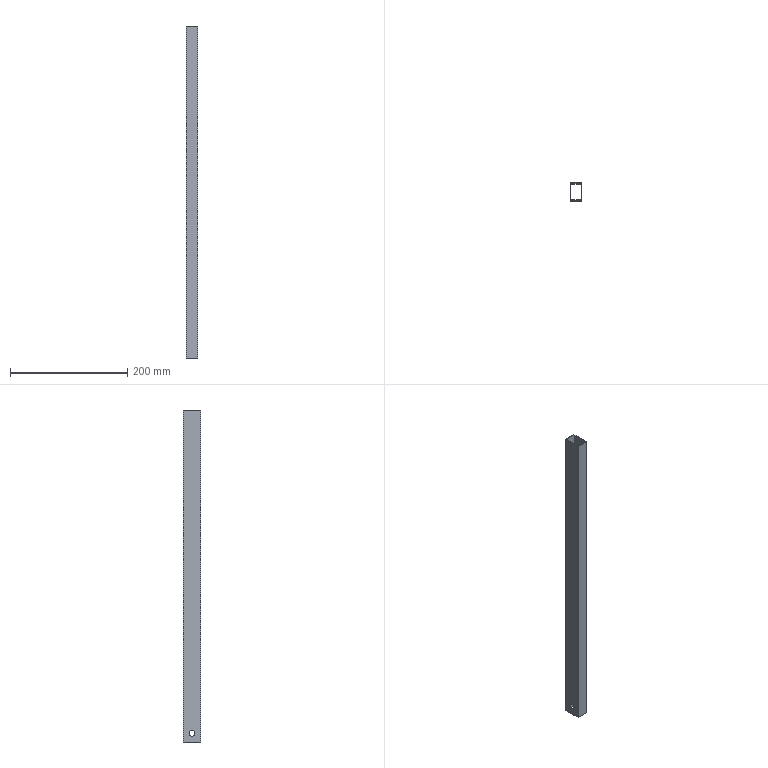Part | SolidWorks | features Extrusion 1, ICE 1 | 1 solid | 14 faces | box 20 x 30 x 566 mm | volume 54179 mm3 | plane 10 | cylinder 4 | commonest cylinder face diameters 10 x4
STEP:
#1=CARTESIAN_POINT('',(1.,-20.,15.));
#2=VERTEX_POINT('',#1);
#3=CARTESIAN_POINT('',(1.,-10.,15.));
#4=VERTEX_POINT('',#3);
#5=CARTESIAN_POINT('',(1.,-15.,15.));
#6=DIRECTION('',(1.,0.,0.));
#7=DIRECTION('',(0.,1.,0.));
#8=AXIS2_PLACEMENT_3D('',#5,#6,#7);
#9=CIRCLE('',#8,5.);
#10=EDGE_CURVE('',#2,#4,#9,.T.);
#11=ORIENTED_EDGE('',*,*,#10,.T.);
#12=CARTESIAN_POINT('',(0.,-10.,15.));
#13=VERTEX_POINT('',#12);
#14=CARTESIAN_POINT('',(20.,-10.,15.));
#15=DIRECTION('',(-1.,0.,0.));
#16=VECTOR('',#15,1000.);
#17=LINE('',#14,#16);
#18=EDGE_CURVE('',#4,#13,#17,.T.);
#19=ORIENTED_EDGE('',*,*,#18,.T.);
#20=CARTESIAN_POINT('',(0.,-20.,15.));
#21=VERTEX_POINT('',#20);
#22=CARTESIAN_POINT('',(0.,-15.,15.));
#23=DIRECTION('',(-1.,0.,0.));
#24=DIRECTION('',(0.,-1.,0.));
#25=AXIS2_PLACEMENT_3D('',#22,#23,#24);
#26=CIRCLE('',#25,5.);
#27=EDGE_CURVE('',#13,#21,#26,.T.);
#28=ORIENTED_EDGE('',*,*,#27,.T.);
#29=CARTESIAN_POINT('',(20.,-20.,15.));
#30=DIRECTION('',(-1.,0.,0.));
#31=VECTOR('',#30,1000.);
#32=LINE('',#29,#31);
#33=EDGE_CURVE('',#2,#21,#32,.T.);
#34=ORIENTED_EDGE('',*,*,#33,.F.);
#35=EDGE_LOOP('',(#11,#19,#28,#34));
#36=FACE_OUTER_BOUND('',#35,.T.);
#37=CARTESIAN_POINT('',(20.,-15.,15.));
#38=DIRECTION('',(-1.,0.,0.));
#39=DIRECTION('',(0.,-1.,0.));
#40=AXIS2_PLACEMENT_3D('',#37,#38,#39);
#41=CYLINDRICAL_SURFACE('',#40,5.);
#42=ADVANCED_FACE('',(#36),#41,.F.);
#43=CARTESIAN_POINT('',(20.,-10.,15.));
#44=VERTEX_POINT('',#43);
#45=CARTESIAN_POINT('',(20.,-20.,15.));
#46=VERTEX_POINT('',#45);
#47=CARTESIAN_POINT('',(20.,-15.,15.));
#48=DIRECTION('',(-1.,0.,0.));
#49=DIRECTION('',(0.,-1.,0.));
#50=AXIS2_PLACEMENT_3D('',#47,#48,#49);
#51=CIRCLE('',#50,5.);
#52=EDGE_CURVE('',#44,#46,#51,.T.);
#53=ORIENTED_EDGE('',*,*,#52,.F.);
#54=CARTESIAN_POINT('',(19.,-10.,15.));
#55=VERTEX_POINT('',#54);
#56=CARTESIAN_POINT('',(20.,-10.,15.));
#57=DIRECTION('',(-1.,0.,0.));
#58=VECTOR('',#57,1000.);
#59=LINE('',#56,#58);
#60=EDGE_CURVE('',#44,#55,#59,.T.);
#61=ORIENTED_EDGE('',*,*,#60,.T.);
#62=CARTESIAN_POINT('',(19.,-20.,15.));
#63=VERTEX_POINT('',#62);
#64=CARTESIAN_POINT('',(19.,-15.,15.));
#65=DIRECTION('',(-1.,0.,0.));
#66=DIRECTION('',(0.,-1.,0.));
#67=AXIS2_PLACEMENT_3D('',#64,#65,#66);
#68=CIRCLE('',#67,5.);
#69=EDGE_CURVE('',#55,#63,#68,.T.);
#70=ORIENTED_EDGE('',*,*,#69,.T.);
#71=CARTESIAN_POINT('',(20.,-20.,15.));
#72=DIRECTION('',(-1.,0.,0.));
#73=VECTOR('',#72,1000.);
#74=LINE('',#71,#73);
#75=EDGE_CURVE('',#46,#63,#74,.T.);
#76=ORIENTED_EDGE('',*,*,#75,.F.);
#77=EDGE_LOOP('',(#53,#61,#70,#76));
#78=FACE_OUTER_BOUND('',#77,.T.);
#79=CARTESIAN_POINT('',(20.,-15.,15.));
#80=DIRECTION('',(-1.,0.,0.));
#81=DIRECTION('',(0.,-1.,0.));
#82=AXIS2_PLACEMENT_3D('',#79,#80,#81);
#83=CYLINDRICAL_SURFACE('',#82,5.);
#84=ADVANCED_FACE('',(#78),#83,.F.);
#85=CARTESIAN_POINT('',(0.,0.,566.));
#86=VERTEX_POINT('',#85);
#87=CARTESIAN_POINT('',(0.,-30.,566.));
#88=VERTEX_POINT('',#87);
#89=CARTESIAN_POINT('',(0.,0.,566.));
#90=DIRECTION('',(0.,-1.,0.));
#91=VECTOR('',#90,1000.);
#92=LINE('',#89,#91);
#93=EDGE_CURVE('',#86,#88,#92,.T.);
#94=ORIENTED_EDGE('',*,*,#93,.T.);
#95=CARTESIAN_POINT('',(20.,-30.,566.));
#96=VERTEX_POINT('',#95);
#97=CARTESIAN_POINT('',(0.,-30.,566.));
#98=DIRECTION('',(1.,0.,0.));
#99=VECTOR('',#98,1000.);
#100=LINE('',#97,#99);
#101=EDGE_CURVE('',#88,#96,#100,.T.);
#102=ORIENTED_EDGE('',*,*,#101,.T.);
#103=CARTESIAN_POINT('',(20.,0.,566.));
#104=VERTEX_POINT('',#103);
#105=CARTESIAN_POINT('',(20.,0.,566.));
#106=DIRECTION('',(0.,1.,0.));
#107=VECTOR('',#106,1000.);
#108=LINE('',#105,#107);
#109=EDGE_CURVE('',#96,#104,#108,.T.);
#110=ORIENTED_EDGE('',*,*,#109,.T.);
#111=CARTESIAN_POINT('',(0.,0.,566.));
#112=DIRECTION('',(-1.,0.,0.));
#113=VECTOR('',#112,1000.);
#114=LINE('',#111,#113);
#115=EDGE_CURVE('',#104,#86,#114,.T.);
#116=ORIENTED_EDGE('',*,*,#115,.T.);
#117=EDGE_LOOP('',(#94,#102,#110,#116));
#118=FACE_OUTER_BOUND('',#117,.T.);
#119=CARTESIAN_POINT('',(1.,-29.,566.));
#120=VERTEX_POINT('',#119);
#121=CARTESIAN_POINT('',(19.,-29.,566.));
#122=VERTEX_POINT('',#121);
#123=CARTESIAN_POINT('',(1.,-29.,566.));
#124=DIRECTION('',(1.,0.,0.));
#125=VECTOR('',#124,1000.);
#126=LINE('',#123,#125);
#127=EDGE_CURVE('',#120,#122,#126,.T.);
#128=ORIENTED_EDGE('',*,*,#127,.F.);
#129=CARTESIAN_POINT('',(1.,-1.,566.));
#130=VERTEX_POINT('',#129);
#131=CARTESIAN_POINT('',(1.,-1.,566.));
#132=DIRECTION('',(0.,-1.,0.));
#133=VECTOR('',#132,1000.);
#134=LINE('',#131,#133);
#135=EDGE_CURVE('',#130,#120,#134,.T.);
#136=ORIENTED_EDGE('',*,*,#135,.F.);
#137=CARTESIAN_POINT('',(19.,-1.,566.));
#138=VERTEX_POINT('',#137);
#139=CARTESIAN_POINT('',(1.,-1.,566.));
#140=DIRECTION('',(-1.,0.,0.));
#141=VECTOR('',#140,1000.);
#142=LINE('',#139,#141);
#143=EDGE_CURVE('',#138,#130,#142,.T.);
#144=ORIENTED_EDGE('',*,*,#143,.F.);
#145=CARTESIAN_POINT('',(19.,-1.,566.));
#146=DIRECTION('',(0.,1.,0.));
#147=VECTOR('',#146,1000.);
#148=LINE('',#145,#147);
#149=EDGE_CURVE('',#122,#138,#148,.T.);
#150=ORIENTED_EDGE('',*,*,#149,.F.);
#151=EDGE_LOOP('',(#128,#136,#144,#150));
#152=FACE_BOUND('',#151,.T.);
#153=CARTESIAN_POINT('',(0.,0.,566.));
#154=DIRECTION('',(0.,0.,1.));
#155=DIRECTION('',(1.,0.,0.));
#156=AXIS2_PLACEMENT_3D('',#153,#154,#155);
#157=PLANE('',#156);
#158=ADVANCED_FACE('',(#118,#152),#157,.T.);
#159=CARTESIAN_POINT('',(0.,0.,0.));
#160=VERTEX_POINT('',#159);
#161=CARTESIAN_POINT('',(0.,-30.,0.));
#162=VERTEX_POINT('',#161);
#163=CARTESIAN_POINT('',(0.,0.,0.));
#164=DIRECTION('',(0.,-1.,0.));
#165=VECTOR('',#164,1000.);
#166=LINE('',#163,#165);
#167=EDGE_CURVE('',#160,#162,#166,.T.);
#168=ORIENTED_EDGE('',*,*,#167,.F.);
#169=CARTESIAN_POINT('',(20.,0.,0.));
#170=VERTEX_POINT('',#169);
#171=CARTESIAN_POINT('',(0.,0.,0.));
#172=DIRECTION('',(-1.,0.,0.));
#173=VECTOR('',#172,1000.);
#174=LINE('',#171,#173);
#175=EDGE_CURVE('',#170,#160,#174,.T.);
#176=ORIENTED_EDGE('',*,*,#175,.F.);
#177=CARTESIAN_POINT('',(20.,-30.,0.));
#178=VERTEX_POINT('',#177);
#179=CARTESIAN_POINT('',(20.,0.,0.));
#180=DIRECTION('',(0.,1.,0.));
#181=VECTOR('',#180,1000.);
#182=LINE('',#179,#181);
#183=EDGE_CURVE('',#178,#170,#182,.T.);
#184=ORIENTED_EDGE('',*,*,#183,.F.);
#185=CARTESIAN_POINT('',(0.,-30.,0.));
#186=DIRECTION('',(1.,0.,0.));
#187=VECTOR('',#186,1000.);
#188=LINE('',#185,#187);
#189=EDGE_CURVE('',#162,#178,#188,.T.);
#190=ORIENTED_EDGE('',*,*,#189,.F.);
#191=EDGE_LOOP('',(#168,#176,#184,#190));
#192=FACE_OUTER_BOUND('',#191,.T.);
#193=CARTESIAN_POINT('',(1.,-1.,0.));
#194=VERTEX_POINT('',#193);
#195=CARTESIAN_POINT('',(1.,-29.,0.));
#196=VERTEX_POINT('',#195);
#197=CARTESIAN_POINT('',(1.,-1.,0.));
#198=DIRECTION('',(0.,-1.,0.));
#199=VECTOR('',#198,1000.);
#200=LINE('',#197,#199);
#201=EDGE_CURVE('',#194,#196,#200,.T.);
#202=ORIENTED_EDGE('',*,*,#201,.T.);
#203=CARTESIAN_POINT('',(19.,-29.,0.));
#204=VERTEX_POINT('',#203);
#205=CARTESIAN_POINT('',(1.,-29.,0.));
#206=DIRECTION('',(1.,0.,0.));
#207=VECTOR('',#206,1000.);
#208=LINE('',#205,#207);
#209=EDGE_CURVE('',#196,#204,#208,.T.);
#210=ORIENTED_EDGE('',*,*,#209,.T.);
#211=CARTESIAN_POINT('',(19.,-1.,0.));
#212=VERTEX_POINT('',#211);
#213=CARTESIAN_POINT('',(19.,-1.,0.));
#214=DIRECTION('',(0.,1.,0.));
#215=VECTOR('',#214,1000.);
#216=LINE('',#213,#215);
#217=EDGE_CURVE('',#204,#212,#216,.T.);
#218=ORIENTED_EDGE('',*,*,#217,.T.);
#219=CARTESIAN_POINT('',(1.,-1.,0.));
#220=DIRECTION('',(-1.,0.,0.));
#221=VECTOR('',#220,1000.);
#222=LINE('',#219,#221);
#223=EDGE_CURVE('',#212,#194,#222,.T.);
#224=ORIENTED_EDGE('',*,*,#223,.T.);
#225=EDGE_LOOP('',(#202,#210,#218,#224));
#226=FACE_BOUND('',#225,.T.);
#227=CARTESIAN_POINT('',(0.,0.,0.));
#228=DIRECTION('',(0.,0.,1.));
#229=DIRECTION('',(1.,0.,0.));
#230=AXIS2_PLACEMENT_3D('',#227,#228,#229);
#231=PLANE('',#230);
#232=ADVANCED_FACE('',(#192,#226),#231,.F.);
#233=CARTESIAN_POINT('',(0.,-15.,15.));
#234=DIRECTION('',(-1.,0.,0.));
#235=DIRECTION('',(0.,-1.,0.));
#236=AXIS2_PLACEMENT_3D('',#233,#234,#235);
#237=CIRCLE('',#236,5.);
#238=EDGE_CURVE('',#21,#13,#237,.T.);
#239=ORIENTED_EDGE('',*,*,#238,.F.);
#240=ORIENTED_EDGE('',*,*,#27,.F.);
#241=EDGE_LOOP('',(#239,#240));
#242=FACE_BOUND('',#241,.T.);
#243=ORIENTED_EDGE('',*,*,#167,.T.);
#244=CARTESIAN_POINT('',(0.,-30.,566.));
#245=DIRECTION('',(0.,0.,-1.));
#246=VECTOR('',#245,1000.);
#247=LINE('',#244,#246);
#248=EDGE_CURVE('',#88,#162,#247,.T.);
#249=ORIENTED_EDGE('',*,*,#248,.F.);
#250=ORIENTED_EDGE('',*,*,#93,.F.);
#251=CARTESIAN_POINT('',(0.,0.,566.));
#252=DIRECTION('',(0.,0.,-1.));
#253=VECTOR('',#252,1000.);
#254=LINE('',#251,#253);
#255=EDGE_CURVE('',#86,#160,#254,.T.);
#256=ORIENTED_EDGE('',*,*,#255,.T.);
#257=EDGE_LOOP('',(#243,#249,#250,#256));
#258=FACE_OUTER_BOUND('',#257,.T.);
#259=CARTESIAN_POINT('',(0.,0.,566.));
#260=DIRECTION('',(1.,0.,0.));
#261=DIRECTION('',(0.,1.,0.));
#262=AXIS2_PLACEMENT_3D('',#259,#260,#261);
#263=PLANE('',#262);
#264=ADVANCED_FACE('',(#242,#258),#263,.F.);
#265=ORIENTED_EDGE('',*,*,#189,.T.);
#266=CARTESIAN_POINT('',(20.,-30.,566.));
#267=DIRECTION('',(0.,0.,-1.));
#268=VECTOR('',#267,1000.);
#269=LINE('',#266,#268);
#270=EDGE_CURVE('',#96,#178,#269,.T.);
#271=ORIENTED_EDGE('',*,*,#270,.F.);
#272=ORIENTED_EDGE('',*,*,#101,.F.);
#273=ORIENTED_EDGE('',*,*,#248,.T.);
#274=EDGE_LOOP('',(#265,#271,#272,#273));
#275=FACE_OUTER_BOUND('',#274,.T.);
#276=CARTESIAN_POINT('',(0.,-30.,566.));
#277=DIRECTION('',(0.,1.,0.));
#278=DIRECTION('',(0.,0.,1.));
#279=AXIS2_PLACEMENT_3D('',#276,#277,#278);
#280=PLANE('',#279);
#281=ADVANCED_FACE('',(#275),#280,.F.);
#282=CARTESIAN_POINT('',(20.,-15.,15.));
#283=DIRECTION('',(-1.,0.,0.));
#284=DIRECTION('',(0.,-1.,0.));
#285=AXIS2_PLACEMENT_3D('',#282,#283,#284);
#286=CIRCLE('',#285,5.);
#287=EDGE_CURVE('',#46,#44,#286,.T.);
#288=ORIENTED_EDGE('',*,*,#287,.T.);
#289=ORIENTED_EDGE('',*,*,#52,.T.);
#290=EDGE_LOOP('',(#288,#289));
#291=FACE_BOUND('',#290,.T.);
#292=ORIENTED_EDGE('',*,*,#183,.T.);
#293=CARTESIAN_POINT('',(20.,0.,566.));
#294=DIRECTION('',(0.,0.,-1.));
#295=VECTOR('',#294,1000.);
#296=LINE('',#293,#295);
#297=EDGE_CURVE('',#104,#170,#296,.T.);
#298=ORIENTED_EDGE('',*,*,#297,.F.);
#299=ORIENTED_EDGE('',*,*,#109,.F.);
#300=ORIENTED_EDGE('',*,*,#270,.T.);
#301=EDGE_LOOP('',(#292,#298,#299,#300));
#302=FACE_OUTER_BOUND('',#301,.T.);
#303=CARTESIAN_POINT('',(20.,0.,566.));
#304=DIRECTION('',(-1.,0.,0.));
#305=DIRECTION('',(0.,-1.,0.));
#306=AXIS2_PLACEMENT_3D('',#303,#304,#305);
#307=PLANE('',#306);
#308=ADVANCED_FACE('',(#291,#302),#307,.F.);
#309=ORIENTED_EDGE('',*,*,#175,.T.);
#310=ORIENTED_EDGE('',*,*,#255,.F.);
#311=ORIENTED_EDGE('',*,*,#115,.F.);
#312=ORIENTED_EDGE('',*,*,#297,.T.);
#313=EDGE_LOOP('',(#309,#310,#311,#312));
#314=FACE_OUTER_BOUND('',#313,.T.);
#315=CARTESIAN_POINT('',(0.,0.,566.));
#316=DIRECTION('',(0.,-1.,0.));
#317=DIRECTION('',(0.,0.,-1.));
#318=AXIS2_PLACEMENT_3D('',#315,#316,#317);
#319=PLANE('',#318);
#320=ADVANCED_FACE('',(#314),#319,.F.);
#321=ORIENTED_EDGE('',*,*,#10,.F.);
#322=CARTESIAN_POINT('',(1.,-15.,15.));
#323=DIRECTION('',(1.,0.,0.));
#324=DIRECTION('',(0.,1.,0.));
#325=AXIS2_PLACEMENT_3D('',#322,#323,#324);
#326=CIRCLE('',#325,5.);
#327=EDGE_CURVE('',#4,#2,#326,.T.);
#328=ORIENTED_EDGE('',*,*,#327,.F.);
#329=EDGE_LOOP('',(#321,#328));
#330=FACE_BOUND('',#329,.T.);
#331=ORIENTED_EDGE('',*,*,#201,.F.);
#332=CARTESIAN_POINT('',(1.,-1.,566.));
#333=DIRECTION('',(0.,0.,-1.));
#334=VECTOR('',#333,1000.);
#335=LINE('',#332,#334);
#336=EDGE_CURVE('',#130,#194,#335,.T.);
#337=ORIENTED_EDGE('',*,*,#336,.F.);
#338=ORIENTED_EDGE('',*,*,#135,.T.);
#339=CARTESIAN_POINT('',(1.,-29.,566.));
#340=DIRECTION('',(0.,0.,-1.));
#341=VECTOR('',#340,1000.);
#342=LINE('',#339,#341);
#343=EDGE_CURVE('',#120,#196,#342,.T.);
#344=ORIENTED_EDGE('',*,*,#343,.T.);
#345=EDGE_LOOP('',(#331,#337,#338,#344));
#346=FACE_OUTER_BOUND('',#345,.T.);
#347=CARTESIAN_POINT('',(1.,-1.,566.));
#348=DIRECTION('',(1.,0.,0.));
#349=DIRECTION('',(0.,1.,0.));
#350=AXIS2_PLACEMENT_3D('',#347,#348,#349);
#351=PLANE('',#350);
#352=ADVANCED_FACE('',(#330,#346),#351,.T.);
#353=ORIENTED_EDGE('',*,*,#209,.F.);
#354=ORIENTED_EDGE('',*,*,#343,.F.);
#355=ORIENTED_EDGE('',*,*,#127,.T.);
#356=CARTESIAN_POINT('',(19.,-29.,566.));
#357=DIRECTION('',(0.,0.,-1.));
#358=VECTOR('',#357,1000.);
#359=LINE('',#356,#358);
#360=EDGE_CURVE('',#122,#204,#359,.T.);
#361=ORIENTED_EDGE('',*,*,#360,.T.);
#362=EDGE_LOOP('',(#353,#354,#355,#361));
#363=FACE_OUTER_BOUND('',#362,.T.);
#364=CARTESIAN_POINT('',(1.,-29.,566.));
#365=DIRECTION('',(0.,1.,0.));
#366=DIRECTION('',(0.,0.,1.));
#367=AXIS2_PLACEMENT_3D('',#364,#365,#366);
#368=PLANE('',#367);
#369=ADVANCED_FACE('',(#363),#368,.T.);
#370=CARTESIAN_POINT('',(19.,-15.,15.));
#371=DIRECTION('',(-1.,0.,0.));
#372=DIRECTION('',(0.,-1.,0.));
#373=AXIS2_PLACEMENT_3D('',#370,#371,#372);
#374=CIRCLE('',#373,5.);
#375=EDGE_CURVE('',#63,#55,#374,.T.);
#376=ORIENTED_EDGE('',*,*,#375,.F.);
#377=ORIENTED_EDGE('',*,*,#69,.F.);
#378=EDGE_LOOP('',(#376,#377));
#379=FACE_BOUND('',#378,.T.);
#380=ORIENTED_EDGE('',*,*,#217,.F.);
#381=ORIENTED_EDGE('',*,*,#360,.F.);
#382=ORIENTED_EDGE('',*,*,#149,.T.);
#383=CARTESIAN_POINT('',(19.,-1.,566.));
#384=DIRECTION('',(0.,0.,-1.));
#385=VECTOR('',#384,1000.);
#386=LINE('',#383,#385);
#387=EDGE_CURVE('',#138,#212,#386,.T.);
#388=ORIENTED_EDGE('',*,*,#387,.T.);
#389=EDGE_LOOP('',(#380,#381,#382,#388));
#390=FACE_OUTER_BOUND('',#389,.T.);
#391=CARTESIAN_POINT('',(19.,-1.,566.));
#392=DIRECTION('',(-1.,0.,0.));
#393=DIRECTION('',(0.,-1.,0.));
#394=AXIS2_PLACEMENT_3D('',#391,#392,#393);
#395=PLANE('',#394);
#396=ADVANCED_FACE('',(#379,#390),#395,.T.);
#397=ORIENTED_EDGE('',*,*,#223,.F.);
#398=ORIENTED_EDGE('',*,*,#387,.F.);
#399=ORIENTED_EDGE('',*,*,#143,.T.);
#400=ORIENTED_EDGE('',*,*,#336,.T.);
#401=EDGE_LOOP('',(#397,#398,#399,#400));
#402=FACE_OUTER_BOUND('',#401,.T.);
#403=CARTESIAN_POINT('',(1.,-1.,566.));
#404=DIRECTION('',(0.,-1.,0.));
#405=DIRECTION('',(0.,0.,-1.));
#406=AXIS2_PLACEMENT_3D('',#403,#404,#405);
#407=PLANE('',#406);
#408=ADVANCED_FACE('',(#402),#407,.T.);
#409=ORIENTED_EDGE('',*,*,#60,.F.);
#410=ORIENTED_EDGE('',*,*,#287,.F.);
#411=ORIENTED_EDGE('',*,*,#75,.T.);
#412=ORIENTED_EDGE('',*,*,#375,.T.);
#413=EDGE_LOOP('',(#409,#410,#411,#412));
#414=FACE_OUTER_BOUND('',#413,.T.);
#415=CARTESIAN_POINT('',(20.,-15.,15.));
#416=DIRECTION('',(-1.,0.,0.));
#417=DIRECTION('',(0.,-1.,0.));
#418=AXIS2_PLACEMENT_3D('',#415,#416,#417);
#419=CYLINDRICAL_SURFACE('',#418,5.);
#420=ADVANCED_FACE('',(#414),#419,.F.);
#421=ORIENTED_EDGE('',*,*,#18,.F.);
#422=ORIENTED_EDGE('',*,*,#327,.T.);
#423=ORIENTED_EDGE('',*,*,#33,.T.);
#424=ORIENTED_EDGE('',*,*,#238,.T.);
#425=EDGE_LOOP('',(#421,#422,#423,#424));
#426=FACE_OUTER_BOUND('',#425,.T.);
#427=CARTESIAN_POINT('',(20.,-15.,15.));
#428=DIRECTION('',(-1.,0.,0.));
#429=DIRECTION('',(0.,-1.,0.));
#430=AXIS2_PLACEMENT_3D('',#427,#428,#429);
#431=CYLINDRICAL_SURFACE('',#430,5.);
#432=ADVANCED_FACE('',(#426),#431,.F.);
#433=CLOSED_SHELL('',(#42,#84,#158,#232,#264,#281,#308,#320,#352,#369,#396,#408,#420,#432));
#434=MANIFOLD_SOLID_BREP('',#433);
#435=CARTESIAN_POINT('',(0.,0.,0.));
#436=DIRECTION('',(0.,0.,1.));
#437=DIRECTION('',(1.,0.,0.));
#438=AXIS2_PLACEMENT_3D('',#435,#436,#437);
#439=(LENGTH_UNIT()NAMED_UNIT(*)SI_UNIT(.MILLI.,.METRE.));
#440=UNCERTAINTY_MEASURE_WITH_UNIT(LENGTH_MEASURE(0.00001),#439,'','');
#441=(NAMED_UNIT(*)PLANE_ANGLE_UNIT()SI_UNIT($,.RADIAN.));
#442=(NAMED_UNIT(*)SI_UNIT($,.STERADIAN.)SOLID_ANGLE_UNIT());
#443=(GEOMETRIC_REPRESENTATION_CONTEXT(3)GLOBAL_UNCERTAINTY_ASSIGNED_CONTEXT((#440))GLOBAL_UNIT_ASSIGNED_CONTEXT((#439,#441,#442))REPRESENTATION_CONTEXT('',''));
#444=ADVANCED_BREP_SHAPE_REPRESENTATION('',(#434,#438),#443);